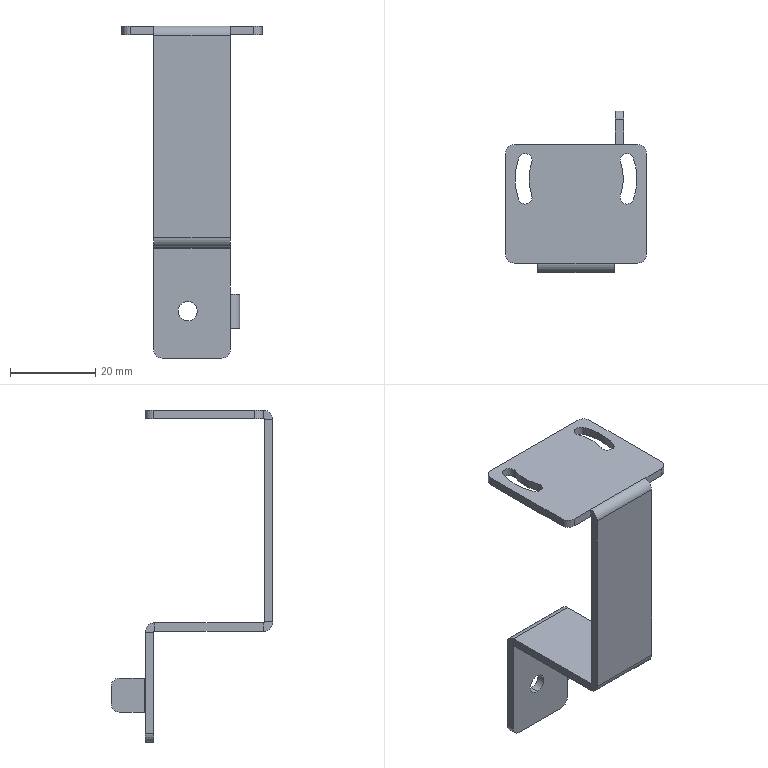Part | STEP file | Photoelectric fixing plate 3 | 1 solid | 64 faces | box 33 x 38 x 78 mm | volume 5566 mm3 | plane 34 | cylinder 30 | commonest cylinder face diameters 4 x8 3.2 x6 0.4 x4 4.4 x4 22.2 x3 28.6 x3